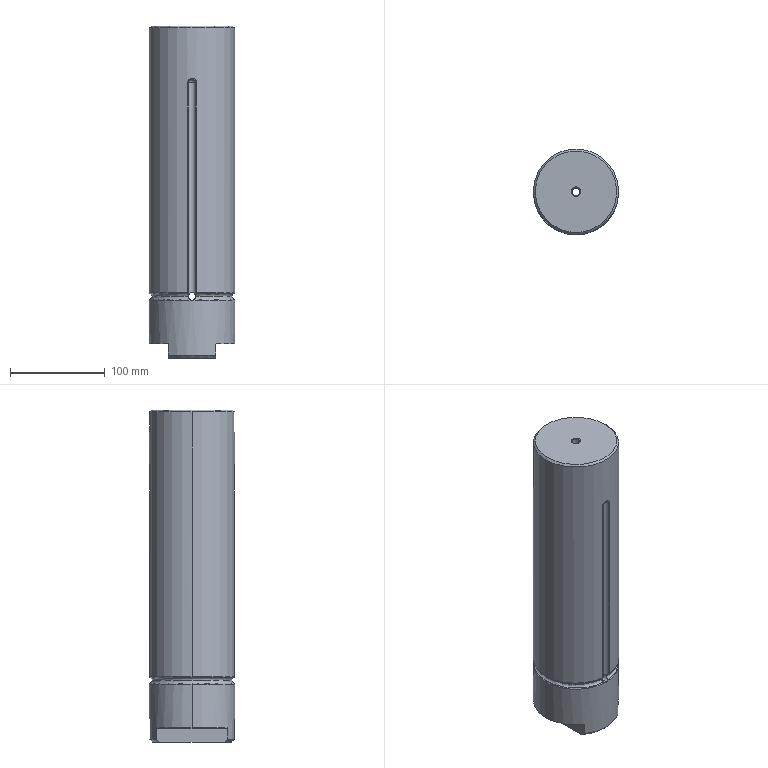Part | SolidWorks | features Fillet 5, ICE 5, 3DProfileFeature 3, HoleWzd 3, Chamfer 2, RevCut 2, Extrusion 1, MirrorPattern 1, RefAxis 1 | 1 solid | 79 faces | box 90 x 90 x 350 mm | volume 2147115 mm3 | cylinder 30 | cone 16 | torus 12 | plane 9 | sphere 6 | spline 6 | commonest cylinder face diameters 8 x10 8.5 x8 2 x4 90 x4 1.6 x2 30 x2